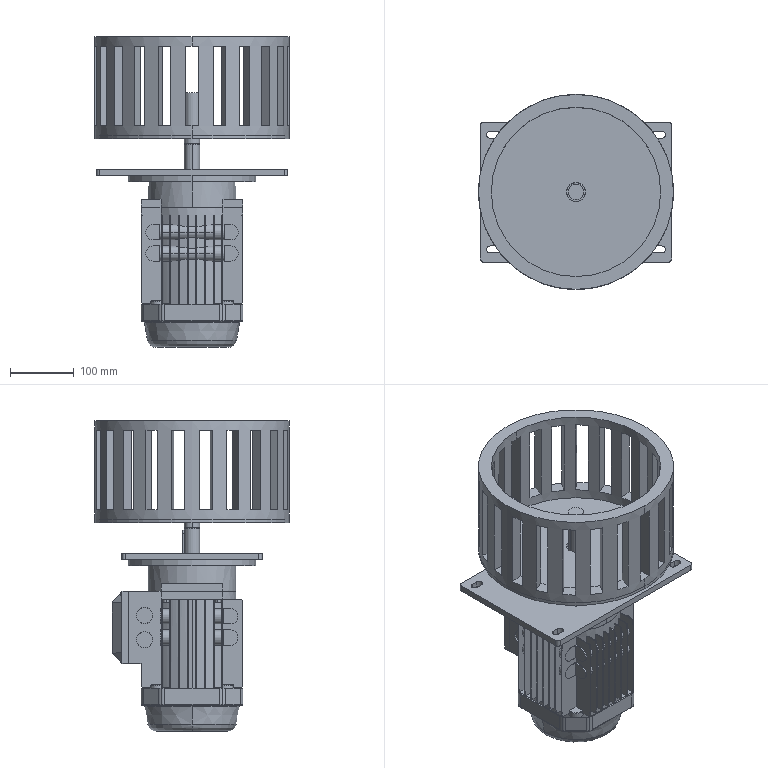Part | SolidWorks | features AEMSimFeature 1 | 6 solids | 1408 faces | box 306 x 306 x 488 mm | volume 7800062 mm3 | plane 1129 | cylinder 219 | torus 44 | cone 14 | sphere 2 | commonest cylinder face diameters 24 x58 6 x20 137.6 x20 10 x18 2 x16 4 x12